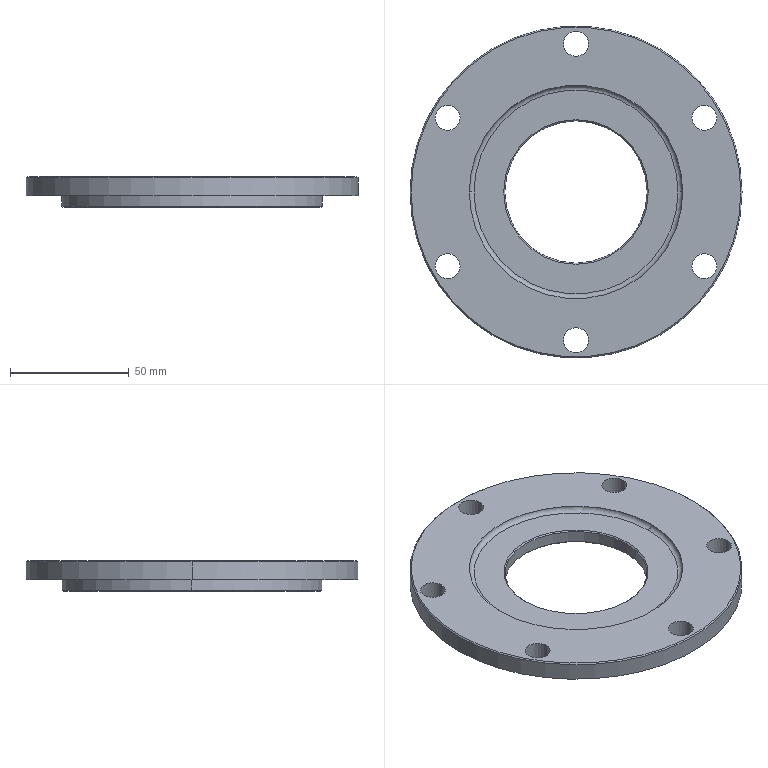Part | SolidWorks | features ICE 3, Chamfer 2, Extrusion 1, Fillet 1 | 1 solid | 35 faces | box 140 x 140 x 13 mm | volume 97648 mm3 | cylinder 20 | cone 8 | plane 5 | torus 2 | commonest cylinder face diameters 10.5 x12 60 x2 100 x2 110 x2 140 x2
STEP:
#1=CARTESIAN_POINT('',(-30.,0.,5.5));
#2=VERTEX_POINT('',#1);
#3=CARTESIAN_POINT('',(30.,0.,5.5));
#4=VERTEX_POINT('',#3);
#5=CARTESIAN_POINT('',(0.,0.,5.5));
#6=DIRECTION('',(0.,0.,1.));
#7=DIRECTION('',(1.,0.,0.));
#8=AXIS2_PLACEMENT_3D('',#5,#6,#7);
#9=CIRCLE('',#8,30.);
#10=EDGE_CURVE('',#2,#4,#9,.T.);
#11=ORIENTED_EDGE('',*,*,#10,.F.);
#12=CARTESIAN_POINT('',(-30.5,0.,6.));
#13=VERTEX_POINT('',#12);
#14=CARTESIAN_POINT('',(-30.,0.,5.5));
#15=DIRECTION('',(-0.7071,0.,0.7071));
#16=VECTOR('',#15,1000.);
#17=LINE('',#14,#16);
#18=EDGE_CURVE('',#2,#13,#17,.T.);
#19=ORIENTED_EDGE('',*,*,#18,.T.);
#20=CARTESIAN_POINT('',(30.5,0.,6.));
#21=VERTEX_POINT('',#20);
#22=CARTESIAN_POINT('',(0.,0.,6.));
#23=DIRECTION('',(0.,0.,-1.));
#24=DIRECTION('',(1.,0.,0.));
#25=AXIS2_PLACEMENT_3D('',#22,#23,#24);
#26=CIRCLE('',#25,30.5);
#27=EDGE_CURVE('',#21,#13,#26,.T.);
#28=ORIENTED_EDGE('',*,*,#27,.F.);
#29=CARTESIAN_POINT('',(30.,0.,5.5));
#30=DIRECTION('',(0.7071,0.,0.7071));
#31=VECTOR('',#30,1000.);
#32=LINE('',#29,#31);
#33=EDGE_CURVE('',#4,#21,#32,.T.);
#34=ORIENTED_EDGE('',*,*,#33,.F.);
#35=EDGE_LOOP('',(#11,#19,#28,#34));
#36=FACE_OUTER_BOUND('',#35,.T.);
#37=CARTESIAN_POINT('',(0.,0.,5.5));
#38=DIRECTION('',(0.,0.,1.));
#39=DIRECTION('',(1.,0.,0.));
#40=AXIS2_PLACEMENT_3D('',#37,#38,#39);
#41=CONICAL_SURFACE('',#40,30.,0.7854);
#42=ADVANCED_FACE('',(#36),#41,.F.);
#43=CARTESIAN_POINT('',(30.,0.,0.5));
#44=VERTEX_POINT('',#43);
#45=CARTESIAN_POINT('',(-30.,0.,0.5));
#46=VERTEX_POINT('',#45);
#47=CARTESIAN_POINT('',(0.,0.,0.5));
#48=DIRECTION('',(0.,0.,-1.));
#49=DIRECTION('',(1.,0.,0.));
#50=AXIS2_PLACEMENT_3D('',#47,#48,#49);
#51=CIRCLE('',#50,30.);
#52=EDGE_CURVE('',#44,#46,#51,.T.);
#53=ORIENTED_EDGE('',*,*,#52,.F.);
#54=CARTESIAN_POINT('',(30.5,0.,0.));
#55=VERTEX_POINT('',#54);
#56=CARTESIAN_POINT('',(30.5,0.,0.));
#57=DIRECTION('',(0.7071,0.,-0.7071));
#58=VECTOR('',#57,1000.);
#59=LINE('',#56,#58);
#60=EDGE_CURVE('',#44,#55,#59,.T.);
#61=ORIENTED_EDGE('',*,*,#60,.T.);
#62=CARTESIAN_POINT('',(-30.5,0.,0.));
#63=VERTEX_POINT('',#62);
#64=CARTESIAN_POINT('',(0.,0.,0.));
#65=DIRECTION('',(0.,0.,1.));
#66=DIRECTION('',(1.,0.,0.));
#67=AXIS2_PLACEMENT_3D('',#64,#65,#66);
#68=CIRCLE('',#67,30.5);
#69=EDGE_CURVE('',#63,#55,#68,.T.);
#70=ORIENTED_EDGE('',*,*,#69,.F.);
#71=CARTESIAN_POINT('',(-30.5,0.,0.));
#72=DIRECTION('',(-0.7071,0.,-0.7071));
#73=VECTOR('',#72,1000.);
#74=LINE('',#71,#73);
#75=EDGE_CURVE('',#46,#63,#74,.T.);
#76=ORIENTED_EDGE('',*,*,#75,.F.);
#77=EDGE_LOOP('',(#53,#61,#70,#76));
#78=FACE_OUTER_BOUND('',#77,.T.);
#79=CARTESIAN_POINT('',(0.,0.,0.));
#80=DIRECTION('',(0.,0.,-1.));
#81=DIRECTION('',(-1.,0.,0.));
#82=AXIS2_PLACEMENT_3D('',#79,#80,#81);
#83=CONICAL_SURFACE('',#82,30.5,0.7854);
#84=ADVANCED_FACE('',(#78),#83,.F.);
#85=ORIENTED_EDGE('',*,*,#52,.T.);
#86=CARTESIAN_POINT('',(-30.,0.,-4.));
#87=DIRECTION('',(0.,0.,1.));
#88=VECTOR('',#87,1000.);
#89=LINE('',#86,#88);
#90=EDGE_CURVE('',#46,#2,#89,.T.);
#91=ORIENTED_EDGE('',*,*,#90,.T.);
#92=ORIENTED_EDGE('',*,*,#10,.T.);
#93=CARTESIAN_POINT('',(30.,0.,-4.));
#94=DIRECTION('',(0.,0.,1.));
#95=VECTOR('',#94,1000.);
#96=LINE('',#93,#95);
#97=EDGE_CURVE('',#44,#4,#96,.T.);
#98=ORIENTED_EDGE('',*,*,#97,.F.);
#99=EDGE_LOOP('',(#85,#91,#92,#98));
#100=FACE_OUTER_BOUND('',#99,.T.);
#101=CARTESIAN_POINT('',(0.,0.,-4.));
#102=DIRECTION('',(0.,0.,1.));
#103=DIRECTION('',(1.,0.,0.));
#104=AXIS2_PLACEMENT_3D('',#101,#102,#103);
#105=CYLINDRICAL_SURFACE('',#104,30.);
#106=ADVANCED_FACE('',(#100),#105,.F.);
#107=CARTESIAN_POINT('',(-43.,0.,6.));
#108=VERTEX_POINT('',#107);
#109=CARTESIAN_POINT('',(43.,0.,6.));
#110=VERTEX_POINT('',#109);
#111=CARTESIAN_POINT('',(0.,0.,6.));
#112=DIRECTION('',(0.,0.,1.));
#113=DIRECTION('',(1.,0.,0.));
#114=AXIS2_PLACEMENT_3D('',#111,#112,#113);
#115=CIRCLE('',#114,43.);
#116=EDGE_CURVE('',#108,#110,#115,.T.);
#117=ORIENTED_EDGE('',*,*,#116,.F.);
#118=CARTESIAN_POINT('',(-45.,0.,8.));
#119=VERTEX_POINT('',#118);
#120=CARTESIAN_POINT('',(-43.,0.,8.));
#121=DIRECTION('',(0.,1.,0.));
#122=DIRECTION('',(-1.,0.,0.));
#123=AXIS2_PLACEMENT_3D('',#120,#121,#122);
#124=CIRCLE('',#123,2.);
#125=EDGE_CURVE('',#108,#119,#124,.T.);
#126=ORIENTED_EDGE('',*,*,#125,.T.);
#127=CARTESIAN_POINT('',(45.,0.,8.));
#128=VERTEX_POINT('',#127);
#129=CARTESIAN_POINT('',(0.,0.,8.));
#130=DIRECTION('',(0.,0.,1.));
#131=DIRECTION('',(1.,0.,0.));
#132=AXIS2_PLACEMENT_3D('',#129,#130,#131);
#133=CIRCLE('',#132,45.);
#134=EDGE_CURVE('',#119,#128,#133,.T.);
#135=ORIENTED_EDGE('',*,*,#134,.T.);
#136=CARTESIAN_POINT('',(43.,0.,8.));
#137=DIRECTION('',(0.,-1.,0.));
#138=DIRECTION('',(0.,0.,-1.));
#139=AXIS2_PLACEMENT_3D('',#136,#137,#138);
#140=CIRCLE('',#139,2.);
#141=EDGE_CURVE('',#110,#128,#140,.T.);
#142=ORIENTED_EDGE('',*,*,#141,.F.);
#143=EDGE_LOOP('',(#117,#126,#135,#142));
#144=FACE_OUTER_BOUND('',#143,.T.);
#145=CARTESIAN_POINT('',(0.,0.,8.));
#146=DIRECTION('',(0.,0.,1.));
#147=DIRECTION('',(1.,0.,0.));
#148=AXIS2_PLACEMENT_3D('',#145,#146,#147);
#149=TOROIDAL_SURFACE('',#148,43.,2.);
#150=ADVANCED_FACE('',(#144),#149,.F.);
#151=CARTESIAN_POINT('',(69.5,0.,8.));
#152=VERTEX_POINT('',#151);
#153=CARTESIAN_POINT('',(-69.5,0.,8.));
#154=VERTEX_POINT('',#153);
#155=CARTESIAN_POINT('',(0.,0.,8.));
#156=DIRECTION('',(0.,0.,1.));
#157=DIRECTION('',(1.,0.,0.));
#158=AXIS2_PLACEMENT_3D('',#155,#156,#157);
#159=CIRCLE('',#158,69.5);
#160=EDGE_CURVE('',#152,#154,#159,.T.);
#161=ORIENTED_EDGE('',*,*,#160,.F.);
#162=CARTESIAN_POINT('',(70.,0.,7.5));
#163=VERTEX_POINT('',#162);
#164=CARTESIAN_POINT('',(69.5,0.,8.));
#165=DIRECTION('',(0.7071,0.,-0.7071));
#166=VECTOR('',#165,1000.);
#167=LINE('',#164,#166);
#168=EDGE_CURVE('',#152,#163,#167,.T.);
#169=ORIENTED_EDGE('',*,*,#168,.T.);
#170=CARTESIAN_POINT('',(-70.,0.,7.5));
#171=VERTEX_POINT('',#170);
#172=CARTESIAN_POINT('',(0.,0.,7.5));
#173=DIRECTION('',(0.,0.,-1.));
#174=DIRECTION('',(1.,0.,0.));
#175=AXIS2_PLACEMENT_3D('',#172,#173,#174);
#176=CIRCLE('',#175,70.);
#177=EDGE_CURVE('',#171,#163,#176,.T.);
#178=ORIENTED_EDGE('',*,*,#177,.F.);
#179=CARTESIAN_POINT('',(-69.5,0.,8.));
#180=DIRECTION('',(-0.7071,0.,-0.7071));
#181=VECTOR('',#180,1000.);
#182=LINE('',#179,#181);
#183=EDGE_CURVE('',#154,#171,#182,.T.);
#184=ORIENTED_EDGE('',*,*,#183,.F.);
#185=EDGE_LOOP('',(#161,#169,#178,#184));
#186=FACE_OUTER_BOUND('',#185,.T.);
#187=CARTESIAN_POINT('',(0.,0.,8.));
#188=DIRECTION('',(0.,0.,-1.));
#189=DIRECTION('',(-1.,0.,0.));
#190=AXIS2_PLACEMENT_3D('',#187,#188,#189);
#191=CONICAL_SURFACE('',#190,69.5,0.7854);
#192=ADVANCED_FACE('',(#186),#191,.T.);
#193=CARTESIAN_POINT('',(-54.5,0.,-5.));
#194=VERTEX_POINT('',#193);
#195=CARTESIAN_POINT('',(54.5,0.,-5.));
#196=VERTEX_POINT('',#195);
#197=CARTESIAN_POINT('',(0.,0.,-5.));
#198=DIRECTION('',(0.,0.,-1.));
#199=DIRECTION('',(-1.,0.,0.));
#200=AXIS2_PLACEMENT_3D('',#197,#198,#199);
#201=CIRCLE('',#200,54.5);
#202=EDGE_CURVE('',#194,#196,#201,.T.);
#203=ORIENTED_EDGE('',*,*,#202,.F.);
#204=CARTESIAN_POINT('',(-55.,0.,-4.5));
#205=VERTEX_POINT('',#204);
#206=CARTESIAN_POINT('',(-54.5,0.,-5.));
#207=DIRECTION('',(-0.7071,0.,0.7071));
#208=VECTOR('',#207,1000.);
#209=LINE('',#206,#208);
#210=EDGE_CURVE('',#194,#205,#209,.T.);
#211=ORIENTED_EDGE('',*,*,#210,.T.);
#212=CARTESIAN_POINT('',(55.,0.,-4.5));
#213=VERTEX_POINT('',#212);
#214=CARTESIAN_POINT('',(0.,0.,-4.5));
#215=DIRECTION('',(0.,0.,1.));
#216=DIRECTION('',(-1.,0.,0.));
#217=AXIS2_PLACEMENT_3D('',#214,#215,#216);
#218=CIRCLE('',#217,55.);
#219=EDGE_CURVE('',#213,#205,#218,.T.);
#220=ORIENTED_EDGE('',*,*,#219,.F.);
#221=CARTESIAN_POINT('',(54.5,0.,-5.));
#222=DIRECTION('',(0.7071,0.,0.7071));
#223=VECTOR('',#222,1000.);
#224=LINE('',#221,#223);
#225=EDGE_CURVE('',#196,#213,#224,.T.);
#226=ORIENTED_EDGE('',*,*,#225,.F.);
#227=EDGE_LOOP('',(#203,#211,#220,#226));
#228=FACE_OUTER_BOUND('',#227,.T.);
#229=CARTESIAN_POINT('',(0.,0.,-5.));
#230=DIRECTION('',(0.,0.,1.));
#231=DIRECTION('',(1.,0.,0.));
#232=AXIS2_PLACEMENT_3D('',#229,#230,#231);
#233=CONICAL_SURFACE('',#232,54.5,0.7854);
#234=ADVANCED_FACE('',(#228),#233,.T.);
#235=CARTESIAN_POINT('',(50.,0.,-5.));
#236=VERTEX_POINT('',#235);
#237=CARTESIAN_POINT('',(-50.,0.,-5.));
#238=VERTEX_POINT('',#237);
#239=CARTESIAN_POINT('',(0.,0.,-5.));
#240=DIRECTION('',(0.,0.,-1.));
#241=DIRECTION('',(-1.,0.,0.));
#242=AXIS2_PLACEMENT_3D('',#239,#240,#241);
#243=CIRCLE('',#242,50.);
#244=EDGE_CURVE('',#236,#238,#243,.T.);
#245=ORIENTED_EDGE('',*,*,#244,.T.);
#246=CARTESIAN_POINT('',(-50.,0.,0.));
#247=VERTEX_POINT('',#246);
#248=CARTESIAN_POINT('',(-50.,0.,-5.));
#249=DIRECTION('',(0.,0.,1.));
#250=VECTOR('',#249,1000.);
#251=LINE('',#248,#250);
#252=EDGE_CURVE('',#238,#247,#251,.T.);
#253=ORIENTED_EDGE('',*,*,#252,.T.);
#254=CARTESIAN_POINT('',(50.,0.,0.));
#255=VERTEX_POINT('',#254);
#256=CARTESIAN_POINT('',(0.,0.,0.));
#257=DIRECTION('',(0.,0.,-1.));
#258=DIRECTION('',(-1.,0.,0.));
#259=AXIS2_PLACEMENT_3D('',#256,#257,#258);
#260=CIRCLE('',#259,50.);
#261=EDGE_CURVE('',#255,#247,#260,.T.);
#262=ORIENTED_EDGE('',*,*,#261,.F.);
#263=CARTESIAN_POINT('',(50.,0.,-5.));
#264=DIRECTION('',(0.,0.,1.));
#265=VECTOR('',#264,1000.);
#266=LINE('',#263,#265);
#267=EDGE_CURVE('',#236,#255,#266,.T.);
#268=ORIENTED_EDGE('',*,*,#267,.F.);
#269=EDGE_LOOP('',(#245,#253,#262,#268));
#270=FACE_OUTER_BOUND('',#269,.T.);
#271=CARTESIAN_POINT('',(0.,0.,-5.));
#272=DIRECTION('',(0.,0.,1.));
#273=DIRECTION('',(1.,0.,0.));
#274=AXIS2_PLACEMENT_3D('',#271,#272,#273);
#275=CYLINDRICAL_SURFACE('',#274,50.);
#276=ADVANCED_FACE('',(#270),#275,.F.);
#277=ORIENTED_EDGE('',*,*,#219,.T.);
#278=CARTESIAN_POINT('',(-55.,0.,0.));
#279=VERTEX_POINT('',#278);
#280=CARTESIAN_POINT('',(-55.,0.,-5.));
#281=DIRECTION('',(0.,0.,1.));
#282=VECTOR('',#281,1000.);
#283=LINE('',#280,#282);
#284=EDGE_CURVE('',#205,#279,#283,.T.);
#285=ORIENTED_EDGE('',*,*,#284,.T.);
#286=CARTESIAN_POINT('',(55.,0.,0.));
#287=VERTEX_POINT('',#286);
#288=CARTESIAN_POINT('',(0.,0.,0.));
#289=DIRECTION('',(0.,0.,-1.));
#290=DIRECTION('',(1.,0.,0.));
#291=AXIS2_PLACEMENT_3D('',#288,#289,#290);
#292=CIRCLE('',#291,55.);
#293=EDGE_CURVE('',#279,#287,#292,.T.);
#294=ORIENTED_EDGE('',*,*,#293,.T.);
#295=CARTESIAN_POINT('',(55.,0.,-5.));
#296=DIRECTION('',(0.,0.,1.));
#297=VECTOR('',#296,1000.);
#298=LINE('',#295,#297);
#299=EDGE_CURVE('',#213,#287,#298,.T.);
#300=ORIENTED_EDGE('',*,*,#299,.F.);
#301=EDGE_LOOP('',(#277,#285,#294,#300));
#302=FACE_OUTER_BOUND('',#301,.T.);
#303=CARTESIAN_POINT('',(0.,0.,-5.));
#304=DIRECTION('',(0.,0.,1.));
#305=DIRECTION('',(1.,0.,0.));
#306=AXIS2_PLACEMENT_3D('',#303,#304,#305);
#307=CYLINDRICAL_SURFACE('',#306,55.);
#308=ADVANCED_FACE('',(#302),#307,.T.);
#309=CARTESIAN_POINT('',(-59.377,31.25,8.));
#310=VERTEX_POINT('',#309);
#311=CARTESIAN_POINT('',(-48.877,31.25,8.));
#312=VERTEX_POINT('',#311);
#313=CARTESIAN_POINT('',(-54.127,31.25,8.));
#314=DIRECTION('',(0.,0.,1.));
#315=DIRECTION('',(1.,0.,0.));
#316=AXIS2_PLACEMENT_3D('',#313,#314,#315);
#317=CIRCLE('',#316,5.25);
#318=EDGE_CURVE('',#310,#312,#317,.T.);
#319=ORIENTED_EDGE('',*,*,#318,.T.);
#320=CARTESIAN_POINT('',(-48.877,31.25,0.));
#321=VERTEX_POINT('',#320);
#322=CARTESIAN_POINT('',(-48.877,31.25,8.));
#323=DIRECTION('',(0.,0.,-1.));
#324=VECTOR('',#323,1000.);
#325=LINE('',#322,#324);
#326=EDGE_CURVE('',#312,#321,#325,.T.);
#327=ORIENTED_EDGE('',*,*,#326,.T.);
#328=CARTESIAN_POINT('',(-59.377,31.25,0.));
#329=VERTEX_POINT('',#328);
#330=CARTESIAN_POINT('',(-54.127,31.25,0.));
#331=DIRECTION('',(0.,0.,1.));
#332=DIRECTION('',(1.,0.,0.));
#333=AXIS2_PLACEMENT_3D('',#330,#331,#332);
#334=CIRCLE('',#333,5.25);
#335=EDGE_CURVE('',#329,#321,#334,.T.);
#336=ORIENTED_EDGE('',*,*,#335,.F.);
#337=CARTESIAN_POINT('',(-59.377,31.25,8.));
#338=DIRECTION('',(0.,0.,-1.));
#339=VECTOR('',#338,1000.);
#340=LINE('',#337,#339);
#341=EDGE_CURVE('',#310,#329,#340,.T.);
#342=ORIENTED_EDGE('',*,*,#341,.F.);
#343=EDGE_LOOP('',(#319,#327,#336,#342));
#344=FACE_OUTER_BOUND('',#343,.T.);
#345=CARTESIAN_POINT('',(-54.127,31.25,8.));
#346=DIRECTION('',(0.,0.,-1.));
#347=DIRECTION('',(-1.,0.,0.));
#348=AXIS2_PLACEMENT_3D('',#345,#346,#347);
#349=CYLINDRICAL_SURFACE('',#348,5.25);
#350=ADVANCED_FACE('',(#344),#349,.F.);
#351=CARTESIAN_POINT('',(-59.377,-31.25,8.));
#352=VERTEX_POINT('',#351);
#353=CARTESIAN_POINT('',(-48.877,-31.25,8.));
#354=VERTEX_POINT('',#353);
#355=CARTESIAN_POINT('',(-54.127,-31.25,8.));
#356=DIRECTION('',(0.,0.,1.));
#357=DIRECTION('',(1.,0.,0.));
#358=AXIS2_PLACEMENT_3D('',#355,#356,#357);
#359=CIRCLE('',#358,5.25);
#360=EDGE_CURVE('',#352,#354,#359,.T.);
#361=ORIENTED_EDGE('',*,*,#360,.T.);
#362=CARTESIAN_POINT('',(-48.877,-31.25,0.));
#363=VERTEX_POINT('',#362);
#364=CARTESIAN_POINT('',(-48.877,-31.25,8.));
#365=DIRECTION('',(0.,0.,-1.));
#366=VECTOR('',#365,1000.);
#367=LINE('',#364,#366);
#368=EDGE_CURVE('',#354,#363,#367,.T.);
#369=ORIENTED_EDGE('',*,*,#368,.T.);
#370=CARTESIAN_POINT('',(-59.377,-31.25,0.));
#371=VERTEX_POINT('',#370);
#372=CARTESIAN_POINT('',(-54.127,-31.25,0.));
#373=DIRECTION('',(0.,0.,1.));
#374=DIRECTION('',(1.,0.,0.));
#375=AXIS2_PLACEMENT_3D('',#372,#373,#374);
#376=CIRCLE('',#375,5.25);
#377=EDGE_CURVE('',#371,#363,#376,.T.);
#378=ORIENTED_EDGE('',*,*,#377,.F.);
#379=CARTESIAN_POINT('',(-59.377,-31.25,8.));
#380=DIRECTION('',(0.,0.,-1.));
#381=VECTOR('',#380,1000.);
#382=LINE('',#379,#381);
#383=EDGE_CURVE('',#352,#371,#382,.T.);
#384=ORIENTED_EDGE('',*,*,#383,.F.);
#385=EDGE_LOOP('',(#361,#369,#378,#384));
#386=FACE_OUTER_BOUND('',#385,.T.);
#387=CARTESIAN_POINT('',(-54.127,-31.25,8.));
#388=DIRECTION('',(0.,0.,-1.));
#389=DIRECTION('',(-1.,0.,0.));
#390=AXIS2_PLACEMENT_3D('',#387,#388,#389);
#391=CYLINDRICAL_SURFACE('',#390,5.25);
#392=ADVANCED_FACE('',(#386),#391,.F.);
#393=CARTESIAN_POINT('',(-5.25,-62.5,8.));
#394=VERTEX_POINT('',#393);
#395=CARTESIAN_POINT('',(5.25,-62.5,8.));
#396=VERTEX_POINT('',#395);
#397=CARTESIAN_POINT('',(0.,-62.5,8.));
#398=DIRECTION('',(0.,0.,1.));
#399=DIRECTION('',(1.,0.,0.));
#400=AXIS2_PLACEMENT_3D('',#397,#398,#399);
#401=CIRCLE('',#400,5.25);
#402=EDGE_CURVE('',#394,#396,#401,.T.);
#403=ORIENTED_EDGE('',*,*,#402,.T.);
#404=CARTESIAN_POINT('',(5.25,-62.5,0.));
#405=VERTEX_POINT('',#404);
#406=CARTESIAN_POINT('',(5.25,-62.5,8.));
#407=DIRECTION('',(0.,0.,-1.));
#408=VECTOR('',#407,1000.);
#409=LINE('',#406,#408);
#410=EDGE_CURVE('',#396,#405,#409,.T.);
#411=ORIENTED_EDGE('',*,*,#410,.T.);
#412=CARTESIAN_POINT('',(-5.25,-62.5,0.));
#413=VERTEX_POINT('',#412);
#414=CARTESIAN_POINT('',(0.,-62.5,0.));
#415=DIRECTION('',(0.,0.,1.));
#416=DIRECTION('',(1.,0.,0.));
#417=AXIS2_PLACEMENT_3D('',#414,#415,#416);
#418=CIRCLE('',#417,5.25);
#419=EDGE_CURVE('',#413,#405,#418,.T.);
#420=ORIENTED_EDGE('',*,*,#419,.F.);
#421=CARTESIAN_POINT('',(-5.25,-62.5,8.));
#422=DIRECTION('',(0.,0.,-1.));
#423=VECTOR('',#422,1000.);
#424=LINE('',#421,#423);
#425=EDGE_CURVE('',#394,#413,#424,.T.);
#426=ORIENTED_EDGE('',*,*,#425,.F.);
#427=EDGE_LOOP('',(#403,#411,#420,#426));
#428=FACE_OUTER_BOUND('',#427,.T.);
#429=CARTESIAN_POINT('',(0.,-62.5,8.));
#430=DIRECTION('',(0.,0.,-1.));
#431=DIRECTION('',(-1.,0.,0.));
#432=AXIS2_PLACEMENT_3D('',#429,#430,#431);
#433=CYLINDRICAL_SURFACE('',#432,5.25);
#434=ADVANCED_FACE('',(#428),#433,.F.);
#435=CARTESIAN_POINT('',(48.877,-31.25,8.));
#436=VERTEX_POINT('',#435);
#437=CARTESIAN_POINT('',(59.377,-31.25,8.));
#438=VERTEX_POINT('',#437);
#439=CARTESIAN_POINT('',(54.127,-31.25,8.));
#440=DIRECTION('',(0.,0.,1.));
#441=DIRECTION('',(1.,0.,0.));
#442=AXIS2_PLACEMENT_3D('',#439,#440,#441);
#443=CIRCLE('',#442,5.25);
#444=EDGE_CURVE('',#436,#438,#443,.T.);
#445=ORIENTED_EDGE('',*,*,#444,.T.);
#446=CARTESIAN_POINT('',(59.377,-31.25,0.));
#447=VERTEX_POINT('',#446);
#448=CARTESIAN_POINT('',(59.377,-31.25,8.));
#449=DIRECTION('',(0.,0.,-1.));
#450=VECTOR('',#449,1000.);
#451=LINE('',#448,#450);
#452=EDGE_CURVE('',#438,#447,#451,.T.);
#453=ORIENTED_EDGE('',*,*,#452,.T.);
#454=CARTESIAN_POINT('',(48.877,-31.25,0.));
#455=VERTEX_POINT('',#454);
#456=CARTESIAN_POINT('',(54.127,-31.25,0.));
#457=DIRECTION('',(0.,0.,1.));
#458=DIRECTION('',(1.,0.,0.));
#459=AXIS2_PLACEMENT_3D('',#456,#457,#458);
#460=CIRCLE('',#459,5.25);
#461=EDGE_CURVE('',#455,#447,#460,.T.);
#462=ORIENTED_EDGE('',*,*,#461,.F.);
#463=CARTESIAN_POINT('',(48.877,-31.25,8.));
#464=DIRECTION('',(0.,0.,-1.));
#465=VECTOR('',#464,1000.);
#466=LINE('',#463,#465);
#467=EDGE_CURVE('',#436,#455,#466,.T.);
#468=ORIENTED_EDGE('',*,*,#467,.F.);
#469=EDGE_LOOP('',(#445,#453,#462,#468));
#470=FACE_OUTER_BOUND('',#469,.T.);
#471=CARTESIAN_POINT('',(54.127,-31.25,8.));
#472=DIRECTION('',(0.,0.,-1.));
#473=DIRECTION('',(-1.,0.,0.));
#474=AXIS2_PLACEMENT_3D('',#471,#472,#473);
#475=CYLINDRICAL_SURFACE('',#474,5.25);
#476=ADVANCED_FACE('',(#470),#475,.F.);
#477=CARTESIAN_POINT('',(48.877,31.25,8.));
#478=VERTEX_POINT('',#477);
#479=CARTESIAN_POINT('',(59.377,31.25,8.));
#480=VERTEX_POINT('',#479);
#481=CARTESIAN_POINT('',(54.127,31.25,8.));
#482=DIRECTION('',(0.,0.,1.));
#483=DIRECTION('',(1.,0.,0.));
#484=AXIS2_PLACEMENT_3D('',#481,#482,#483);
#485=CIRCLE('',#484,5.25);
#486=EDGE_CURVE('',#478,#480,#485,.T.);
#487=ORIENTED_EDGE('',*,*,#486,.T.);
#488=CARTESIAN_POINT('',(59.377,31.25,0.));
#489=VERTEX_POINT('',#488);
#490=CARTESIAN_POINT('',(59.377,31.25,8.));
#491=DIRECTION('',(0.,0.,-1.));
#492=VECTOR('',#491,1000.);
#493=LINE('',#490,#492);
#494=EDGE_CURVE('',#480,#489,#493,.T.);
#495=ORIENTED_EDGE('',*,*,#494,.T.);
#496=CARTESIAN_POINT('',(48.877,31.25,0.));
#497=VERTEX_POINT('',#496);
#498=CARTESIAN_POINT('',(54.127,31.25,0.));
#499=DIRECTION('',(0.,0.,1.));
#500=DIRECTION('',(1.,0.,0.));
#501=AXIS2_PLACEMENT_3D('',#498,#499,#500);
#502=CIRCLE('',#501,5.25);
#503=EDGE_CURVE('',#497,#489,#502,.T.);
#504=ORIENTED_EDGE('',*,*,#503,.F.);
#505=CARTESIAN_POINT('',(48.877,31.25,8.));
#506=DIRECTION('',(0.,0.,-1.));
#507=VECTOR('',#506,1000.);
#508=LINE('',#505,#507);
#509=EDGE_CURVE('',#478,#497,#508,.T.);
#510=ORIENTED_EDGE('',*,*,#509,.F.);
#511=EDGE_LOOP('',(#487,#495,#504,#510));
#512=FACE_OUTER_BOUND('',#511,.T.);
#513=CARTESIAN_POINT('',(54.127,31.25,8.));
#514=DIRECTION('',(0.,0.,-1.));
#515=DIRECTION('',(-1.,0.,0.));
#516=AXIS2_PLACEMENT_3D('',#513,#514,#515);
#517=CYLINDRICAL_SURFACE('',#516,5.25);
#518=ADVANCED_FACE('',(#512),#517,.F.);
#519=CARTESIAN_POINT('',(-5.25,62.5,8.));
#520=VERTEX_POINT('',#519);
#521=CARTESIAN_POINT('',(5.25,62.5,8.));
#522=VERTEX_POINT('',#521);
#523=CARTESIAN_POINT('',(0.,62.5,8.));
#524=DIRECTION('',(0.,0.,1.));
#525=DIRECTION('',(1.,0.,0.));
#526=AXIS2_PLACEMENT_3D('',#523,#524,#525);
#527=CIRCLE('',#526,5.25);
#528=EDGE_CURVE('',#520,#522,#527,.T.);
#529=ORIENTED_EDGE('',*,*,#528,.T.);
#530=CARTESIAN_POINT('',(5.25,62.5,0.));
#531=VERTEX_POINT('',#530);
#532=CARTESIAN_POINT('',(5.25,62.5,8.));
#533=DIRECTION('',(0.,0.,-1.));
#534=VECTOR('',#533,1000.);
#535=LINE('',#532,#534);
#536=EDGE_CURVE('',#522,#531,#535,.T.);
#537=ORIENTED_EDGE('',*,*,#536,.T.);
#538=CARTESIAN_POINT('',(-5.25,62.5,0.));
#539=VERTEX_POINT('',#538);
#540=CARTESIAN_POINT('',(0.,62.5,0.));
#541=DIRECTION('',(0.,0.,1.));
#542=DIRECTION('',(1.,0.,0.));
#543=AXIS2_PLACEMENT_3D('',#540,#541,#542);
#544=CIRCLE('',#543,5.25);
#545=EDGE_CURVE('',#539,#531,#544,.T.);
#546=ORIENTED_EDGE('',*,*,#545,.F.);
#547=CARTESIAN_POINT('',(-5.25,62.5,8.));
#548=DIRECTION('',(0.,0.,-1.));
#549=VECTOR('',#548,1000.);
#550=LINE('',#547,#549);
#551=EDGE_CURVE('',#520,#539,#550,.T.);
#552=ORIENTED_EDGE('',*,*,#551,.F.);
#553=EDGE_LOOP('',(#529,#537,#546,#552));
#554=FACE_OUTER_BOUND('',#553,.T.);
#555=CARTESIAN_POINT('',(0.,62.5,8.));
#556=DIRECTION('',(0.,0.,-1.));
#557=DIRECTION('',(-1.,0.,0.));
#558=AXIS2_PLACEMENT_3D('',#555,#556,#557);
#559=CYLINDRICAL_SURFACE('',#558,5.25);
#560=ADVANCED_FACE('',(#554),#559,.F.);
#561=ORIENTED_EDGE('',*,*,#177,.T.);
#562=CARTESIAN_POINT('',(70.,0.,0.));
#563=VERTEX_POINT('',#562);
#564=CARTESIAN_POINT('',(70.,0.,8.));
#565=DIRECTION('',(0.,0.,-1.));
#566=VECTOR('',#565,1000.);
#567=LINE('',#564,#566);
#568=EDGE_CURVE('',#163,#563,#567,.T.);
#569=ORIENTED_EDGE('',*,*,#568,.T.);
#570=CARTESIAN_POINT('',(-70.,0.,0.));
#571=VERTEX_POINT('',#570);
#572=CARTESIAN_POINT('',(0.,0.,0.));
#573=DIRECTION('',(0.,0.,1.));
#574=DIRECTION('',(1.,0.,0.));
#575=AXIS2_PLACEMENT_3D('',#572,#573,#574);
#576=CIRCLE('',#575,70.);
#577=EDGE_CURVE('',#563,#571,#576,.T.);
#578=ORIENTED_EDGE('',*,*,#577,.T.);
#579=CARTESIAN_POINT('',(-70.,0.,8.));
#580=DIRECTION('',(0.,0.,-1.));
#581=VECTOR('',#580,1000.);
#582=LINE('',#579,#581);
#583=EDGE_CURVE('',#171,#571,#582,.T.);
#584=ORIENTED_EDGE('',*,*,#583,.F.);
#585=EDGE_LOOP('',(#561,#569,#578,#584));
#586=FACE_OUTER_BOUND('',#585,.T.);
#587=CARTESIAN_POINT('',(0.,0.,8.));
#588=DIRECTION('',(0.,0.,-1.));
#589=DIRECTION('',(-1.,0.,0.));
#590=AXIS2_PLACEMENT_3D('',#587,#588,#589);
#591=CYLINDRICAL_SURFACE('',#590,70.);
#592=ADVANCED_FACE('',(#586),#591,.T.);
#593=CARTESIAN_POINT('',(0.,0.,8.));
#594=DIRECTION('',(0.,0.,1.));
#595=DIRECTION('',(1.,0.,0.));
#596=AXIS2_PLACEMENT_3D('',#593,#594,#595);
#597=CIRCLE('',#596,45.);
#598=EDGE_CURVE('',#128,#119,#597,.T.);
#599=ORIENTED_EDGE('',*,*,#598,.F.);
#600=ORIENTED_EDGE('',*,*,#134,.F.);
#601=EDGE_LOOP('',(#599,#600));
#602=FACE_BOUND('',#601,.T.);
#603=CARTESIAN_POINT('',(0.,0.,8.));
#604=DIRECTION('',(0.,0.,1.));
#605=DIRECTION('',(1.,0.,0.));
#606=AXIS2_PLACEMENT_3D('',#603,#604,#605);
#607=CIRCLE('',#606,69.5);
#608=EDGE_CURVE('',#154,#152,#607,.T.);
#609=ORIENTED_EDGE('',*,*,#608,.T.);
#610=ORIENTED_EDGE('',*,*,#160,.T.);
#611=EDGE_LOOP('',(#609,#610));
#612=FACE_OUTER_BOUND('',#611,.T.);
#613=ORIENTED_EDGE('',*,*,#360,.F.);
#614=CARTESIAN_POINT('',(-54.127,-31.25,8.));
#615=DIRECTION('',(0.,0.,1.));
#616=DIRECTION('',(1.,0.,0.));
#617=AXIS2_PLACEMENT_3D('',#614,#615,#616);
#618=CIRCLE('',#617,5.25);
#619=EDGE_CURVE('',#354,#352,#618,.T.);
#620=ORIENTED_EDGE('',*,*,#619,.F.);
#621=EDGE_LOOP('',(#613,#620));
#622=FACE_BOUND('',#621,.T.);
#623=ORIENTED_EDGE('',*,*,#444,.F.);
#624=CARTESIAN_POINT('',(54.127,-31.25,8.));
#625=DIRECTION('',(0.,0.,1.));
#626=DIRECTION('',(1.,0.,0.));
#627=AXIS2_PLACEMENT_3D('',#624,#625,#626);
#628=CIRCLE('',#627,5.25);
#629=EDGE_CURVE('',#438,#436,#628,.T.);
#630=ORIENTED_EDGE('',*,*,#629,.F.);
#631=EDGE_LOOP('',(#623,#630));
#632=FACE_BOUND('',#631,.T.);
#633=ORIENTED_EDGE('',*,*,#528,.F.);
#634=CARTESIAN_POINT('',(0.,62.5,8.));
#635=DIRECTION('',(0.,0.,1.));
#636=DIRECTION('',(1.,0.,0.));
#637=AXIS2_PLACEMENT_3D('',#634,#635,#636);
#638=CIRCLE('',#637,5.25);
#639=EDGE_CURVE('',#522,#520,#638,.T.);
#640=ORIENTED_EDGE('',*,*,#639,.F.);
#641=EDGE_LOOP('',(#633,#640));
#642=FACE_BOUND('',#641,.T.);
#643=ORIENTED_EDGE('',*,*,#486,.F.);
#644=CARTESIAN_POINT('',(54.127,31.25,8.));
#645=DIRECTION('',(0.,0.,1.));
#646=DIRECTION('',(1.,0.,0.));
#647=AXIS2_PLACEMENT_3D('',#644,#645,#646);
#648=CIRCLE('',#647,5.25);
#649=EDGE_CURVE('',#480,#478,#648,.T.);
#650=ORIENTED_EDGE('',*,*,#649,.F.);
#651=EDGE_LOOP('',(#643,#650));
#652=FACE_BOUND('',#651,.T.);
#653=ORIENTED_EDGE('',*,*,#402,.F.);
#654=CARTESIAN_POINT('',(0.,-62.5,8.));
#655=DIRECTION('',(0.,0.,1.));
#656=DIRECTION('',(1.,0.,0.));
#657=AXIS2_PLACEMENT_3D('',#654,#655,#656);
#658=CIRCLE('',#657,5.25);
#659=EDGE_CURVE('',#396,#394,#658,.T.);
#660=ORIENTED_EDGE('',*,*,#659,.F.);
#661=EDGE_LOOP('',(#653,#660));
#662=FACE_BOUND('',#661,.T.);
#663=ORIENTED_EDGE('',*,*,#318,.F.);
#664=CARTESIAN_POINT('',(-54.127,31.25,8.));
#665=DIRECTION('',(0.,0.,1.));
#666=DIRECTION('',(1.,0.,0.));
#667=AXIS2_PLACEMENT_3D('',#664,#665,#666);
#668=CIRCLE('',#667,5.25);
#669=EDGE_CURVE('',#312,#310,#668,.T.);
#670=ORIENTED_EDGE('',*,*,#669,.F.);
#671=EDGE_LOOP('',(#663,#670));
#672=FACE_BOUND('',#671,.T.);
#673=CARTESIAN_POINT('',(0.,0.,8.));
#674=DIRECTION('',(0.,0.,1.));
#675=DIRECTION('',(1.,0.,0.));
#676=AXIS2_PLACEMENT_3D('',#673,#674,#675);
#677=PLANE('',#676);
#678=ADVANCED_FACE('',(#602,#612,#622,#632,#642,#652,#662,#672),#677,.T.);
#679=CARTESIAN_POINT('',(0.,0.,0.));
#680=DIRECTION('',(0.,0.,-1.));
#681=DIRECTION('',(1.,0.,0.));
#682=AXIS2_PLACEMENT_3D('',#679,#680,#681);
#683=CIRCLE('',#682,55.);
#684=EDGE_CURVE('',#287,#279,#683,.T.);
#685=ORIENTED_EDGE('',*,*,#684,.F.);
#686=ORIENTED_EDGE('',*,*,#293,.F.);
#687=EDGE_LOOP('',(#685,#686));
#688=FACE_BOUND('',#687,.T.);
#689=CARTESIAN_POINT('',(0.,0.,0.));
#690=DIRECTION('',(0.,0.,1.));
#691=DIRECTION('',(1.,0.,0.));
#692=AXIS2_PLACEMENT_3D('',#689,#690,#691);
#693=CIRCLE('',#692,70.);
#694=EDGE_CURVE('',#571,#563,#693,.T.);
#695=ORIENTED_EDGE('',*,*,#694,.F.);
#696=ORIENTED_EDGE('',*,*,#577,.F.);
#697=EDGE_LOOP('',(#695,#696));
#698=FACE_OUTER_BOUND('',#697,.T.);
#699=ORIENTED_EDGE('',*,*,#545,.T.);
#700=CARTESIAN_POINT('',(0.,62.5,0.));
#701=DIRECTION('',(0.,0.,1.));
#702=DIRECTION('',(1.,0.,0.));
#703=AXIS2_PLACEMENT_3D('',#700,#701,#702);
#704=CIRCLE('',#703,5.25);
#705=EDGE_CURVE('',#531,#539,#704,.T.);
#706=ORIENTED_EDGE('',*,*,#705,.T.);
#707=EDGE_LOOP('',(#699,#706));
#708=FACE_BOUND('',#707,.T.);
#709=ORIENTED_EDGE('',*,*,#503,.T.);
#710=CARTESIAN_POINT('',(54.127,31.25,0.));
#711=DIRECTION('',(0.,0.,1.));
#712=DIRECTION('',(1.,0.,0.));
#713=AXIS2_PLACEMENT_3D('',#710,#711,#712);
#714=CIRCLE('',#713,5.25);
#715=EDGE_CURVE('',#489,#497,#714,.T.);
#716=ORIENTED_EDGE('',*,*,#715,.T.);
#717=EDGE_LOOP('',(#709,#716));
#718=FACE_BOUND('',#717,.T.);
#719=ORIENTED_EDGE('',*,*,#461,.T.);
#720=CARTESIAN_POINT('',(54.127,-31.25,0.));
#721=DIRECTION('',(0.,0.,1.));
#722=DIRECTION('',(1.,0.,0.));
#723=AXIS2_PLACEMENT_3D('',#720,#721,#722);
#724=CIRCLE('',#723,5.25);
#725=EDGE_CURVE('',#447,#455,#724,.T.);
#726=ORIENTED_EDGE('',*,*,#725,.T.);
#727=EDGE_LOOP('',(#719,#726));
#728=FACE_BOUND('',#727,.T.);
#729=ORIENTED_EDGE('',*,*,#419,.T.);
#730=CARTESIAN_POINT('',(0.,-62.5,0.));
#731=DIRECTION('',(0.,0.,1.));
#732=DIRECTION('',(1.,0.,0.));
#733=AXIS2_PLACEMENT_3D('',#730,#731,#732);
#734=CIRCLE('',#733,5.25);
#735=EDGE_CURVE('',#405,#413,#734,.T.);
#736=ORIENTED_EDGE('',*,*,#735,.T.);
#737=EDGE_LOOP('',(#729,#736));
#738=FACE_BOUND('',#737,.T.);
#739=ORIENTED_EDGE('',*,*,#377,.T.);
#740=CARTESIAN_POINT('',(-54.127,-31.25,0.));
#741=DIRECTION('',(0.,0.,1.));
#742=DIRECTION('',(1.,0.,0.));
#743=AXIS2_PLACEMENT_3D('',#740,#741,#742);
#744=CIRCLE('',#743,5.25);
#745=EDGE_CURVE('',#363,#371,#744,.T.);
#746=ORIENTED_EDGE('',*,*,#745,.T.);
#747=EDGE_LOOP('',(#739,#746));
#748=FACE_BOUND('',#747,.T.);
#749=ORIENTED_EDGE('',*,*,#335,.T.);
#750=CARTESIAN_POINT('',(-54.127,31.25,0.));
#751=DIRECTION('',(0.,0.,1.));
#752=DIRECTION('',(1.,0.,0.));
#753=AXIS2_PLACEMENT_3D('',#750,#751,#752);
#754=CIRCLE('',#753,5.25);
#755=EDGE_CURVE('',#321,#329,#754,.T.);
#756=ORIENTED_EDGE('',*,*,#755,.T.);
#757=EDGE_LOOP('',(#749,#756));
#758=FACE_BOUND('',#757,.T.);
#759=CARTESIAN_POINT('',(0.,0.,0.));
#760=DIRECTION('',(0.,0.,1.));
#761=DIRECTION('',(1.,0.,0.));
#762=AXIS2_PLACEMENT_3D('',#759,#760,#761);
#763=PLANE('',#762);
#764=ADVANCED_FACE('',(#688,#698,#708,#718,#728,#738,#748,#758),#763,.F.);
#765=ORIENTED_EDGE('',*,*,#568,.F.);
#766=CARTESIAN_POINT('',(0.,0.,7.5));
#767=DIRECTION('',(0.,0.,-1.));
#768=DIRECTION('',(1.,0.,0.));
#769=AXIS2_PLACEMENT_3D('',#766,#767,#768);
#770=CIRCLE('',#769,70.);
#771=EDGE_CURVE('',#163,#171,#770,.T.);
#772=ORIENTED_EDGE('',*,*,#771,.T.);
#773=ORIENTED_EDGE('',*,*,#583,.T.);
#774=ORIENTED_EDGE('',*,*,#694,.T.);
#775=EDGE_LOOP('',(#765,#772,#773,#774));
#776=FACE_OUTER_BOUND('',#775,.T.);
#777=CARTESIAN_POINT('',(0.,0.,8.));
#778=DIRECTION('',(0.,0.,-1.));
#779=DIRECTION('',(-1.,0.,0.));
#780=AXIS2_PLACEMENT_3D('',#777,#778,#779);
#781=CYLINDRICAL_SURFACE('',#780,70.);
#782=ADVANCED_FACE('',(#776),#781,.T.);
#783=ORIENTED_EDGE('',*,*,#536,.F.);
#784=ORIENTED_EDGE('',*,*,#639,.T.);
#785=ORIENTED_EDGE('',*,*,#551,.T.);
#786=ORIENTED_EDGE('',*,*,#705,.F.);
#787=EDGE_LOOP('',(#783,#784,#785,#786));
#788=FACE_OUTER_BOUND('',#787,.T.);
#789=CARTESIAN_POINT('',(0.,62.5,8.));
#790=DIRECTION('',(0.,0.,-1.));
#791=DIRECTION('',(-1.,0.,0.));
#792=AXIS2_PLACEMENT_3D('',#789,#790,#791);
#793=CYLINDRICAL_SURFACE('',#792,5.25);
#794=ADVANCED_FACE('',(#788),#793,.F.);
#795=ORIENTED_EDGE('',*,*,#494,.F.);
#796=ORIENTED_EDGE('',*,*,#649,.T.);
#797=ORIENTED_EDGE('',*,*,#509,.T.);
#798=ORIENTED_EDGE('',*,*,#715,.F.);
#799=EDGE_LOOP('',(#795,#796,#797,#798));
#800=FACE_OUTER_BOUND('',#799,.T.);
#801=CARTESIAN_POINT('',(54.127,31.25,8.));
#802=DIRECTION('',(0.,0.,-1.));
#803=DIRECTION('',(-1.,0.,0.));
#804=AXIS2_PLACEMENT_3D('',#801,#802,#803);
#805=CYLINDRICAL_SURFACE('',#804,5.25);
#806=ADVANCED_FACE('',(#800),#805,.F.);
#807=ORIENTED_EDGE('',*,*,#452,.F.);
#808=ORIENTED_EDGE('',*,*,#629,.T.);
#809=ORIENTED_EDGE('',*,*,#467,.T.);
#810=ORIENTED_EDGE('',*,*,#725,.F.);
#811=EDGE_LOOP('',(#807,#808,#809,#810));
#812=FACE_OUTER_BOUND('',#811,.T.);
#813=CARTESIAN_POINT('',(54.127,-31.25,8.));
#814=DIRECTION('',(0.,0.,-1.));
#815=DIRECTION('',(-1.,0.,0.));
#816=AXIS2_PLACEMENT_3D('',#813,#814,#815);
#817=CYLINDRICAL_SURFACE('',#816,5.25);
#818=ADVANCED_FACE('',(#812),#817,.F.);
#819=ORIENTED_EDGE('',*,*,#410,.F.);
#820=ORIENTED_EDGE('',*,*,#659,.T.);
#821=ORIENTED_EDGE('',*,*,#425,.T.);
#822=ORIENTED_EDGE('',*,*,#735,.F.);
#823=EDGE_LOOP('',(#819,#820,#821,#822));
#824=FACE_OUTER_BOUND('',#823,.T.);
#825=CARTESIAN_POINT('',(0.,-62.5,8.));
#826=DIRECTION('',(0.,0.,-1.));
#827=DIRECTION('',(-1.,0.,0.));
#828=AXIS2_PLACEMENT_3D('',#825,#826,#827);
#829=CYLINDRICAL_SURFACE('',#828,5.25);
#830=ADVANCED_FACE('',(#824),#829,.F.);
#831=ORIENTED_EDGE('',*,*,#368,.F.);
#832=ORIENTED_EDGE('',*,*,#619,.T.);
#833=ORIENTED_EDGE('',*,*,#383,.T.);
#834=ORIENTED_EDGE('',*,*,#745,.F.);
#835=EDGE_LOOP('',(#831,#832,#833,#834));
#836=FACE_OUTER_BOUND('',#835,.T.);
#837=CARTESIAN_POINT('',(-54.127,-31.25,8.));
#838=DIRECTION('',(0.,0.,-1.));
#839=DIRECTION('',(-1.,0.,0.));
#840=AXIS2_PLACEMENT_3D('',#837,#838,#839);
#841=CYLINDRICAL_SURFACE('',#840,5.25);
#842=ADVANCED_FACE('',(#836),#841,.F.);
#843=ORIENTED_EDGE('',*,*,#326,.F.);
#844=ORIENTED_EDGE('',*,*,#669,.T.);
#845=ORIENTED_EDGE('',*,*,#341,.T.);
#846=ORIENTED_EDGE('',*,*,#755,.F.);
#847=EDGE_LOOP('',(#843,#844,#845,#846));
#848=FACE_OUTER_BOUND('',#847,.T.);
#849=CARTESIAN_POINT('',(-54.127,31.25,8.));
#850=DIRECTION('',(0.,0.,-1.));
#851=DIRECTION('',(-1.,0.,0.));
#852=AXIS2_PLACEMENT_3D('',#849,#850,#851);
#853=CYLINDRICAL_SURFACE('',#852,5.25);
#854=ADVANCED_FACE('',(#848),#853,.F.);
#855=CARTESIAN_POINT('',(0.,0.,-5.));
#856=DIRECTION('',(0.,0.,-1.));
#857=DIRECTION('',(-1.,0.,0.));
#858=AXIS2_PLACEMENT_3D('',#855,#856,#857);
#859=CIRCLE('',#858,54.5);
#860=EDGE_CURVE('',#196,#194,#859,.T.);
#861=ORIENTED_EDGE('',*,*,#860,.T.);
#862=ORIENTED_EDGE('',*,*,#202,.T.);
#863=EDGE_LOOP('',(#861,#862));
#864=FACE_OUTER_BOUND('',#863,.T.);
#865=ORIENTED_EDGE('',*,*,#244,.F.);
#866=CARTESIAN_POINT('',(0.,0.,-5.));
#867=DIRECTION('',(0.,0.,-1.));
#868=DIRECTION('',(-1.,0.,0.));
#869=AXIS2_PLACEMENT_3D('',#866,#867,#868);
#870=CIRCLE('',#869,50.);
#871=EDGE_CURVE('',#238,#236,#870,.T.);
#872=ORIENTED_EDGE('',*,*,#871,.F.);
#873=EDGE_LOOP('',(#865,#872));
#874=FACE_BOUND('',#873,.T.);
#875=CARTESIAN_POINT('',(0.,0.,-5.));
#876=DIRECTION('',(0.,0.,-1.));
#877=DIRECTION('',(-1.,0.,0.));
#878=AXIS2_PLACEMENT_3D('',#875,#876,#877);
#879=PLANE('',#878);
#880=ADVANCED_FACE('',(#864,#874),#879,.T.);
#881=ORIENTED_EDGE('',*,*,#284,.F.);
#882=CARTESIAN_POINT('',(0.,0.,-4.5));
#883=DIRECTION('',(0.,0.,1.));
#884=DIRECTION('',(-1.,0.,0.));
#885=AXIS2_PLACEMENT_3D('',#882,#883,#884);
#886=CIRCLE('',#885,55.);
#887=EDGE_CURVE('',#205,#213,#886,.T.);
#888=ORIENTED_EDGE('',*,*,#887,.T.);
#889=ORIENTED_EDGE('',*,*,#299,.T.);
#890=ORIENTED_EDGE('',*,*,#684,.T.);
#891=EDGE_LOOP('',(#881,#888,#889,#890));
#892=FACE_OUTER_BOUND('',#891,.T.);
#893=CARTESIAN_POINT('',(0.,0.,-5.));
#894=DIRECTION('',(0.,0.,1.));
#895=DIRECTION('',(1.,0.,0.));
#896=AXIS2_PLACEMENT_3D('',#893,#894,#895);
#897=CYLINDRICAL_SURFACE('',#896,55.);
#898=ADVANCED_FACE('',(#892),#897,.T.);
#899=ORIENTED_EDGE('',*,*,#252,.F.);
#900=ORIENTED_EDGE('',*,*,#871,.T.);
#901=ORIENTED_EDGE('',*,*,#267,.T.);
#902=CARTESIAN_POINT('',(0.,0.,0.));
#903=DIRECTION('',(0.,0.,-1.));
#904=DIRECTION('',(-1.,0.,0.));
#905=AXIS2_PLACEMENT_3D('',#902,#903,#904);
#906=CIRCLE('',#905,50.);
#907=EDGE_CURVE('',#247,#255,#906,.T.);
#908=ORIENTED_EDGE('',*,*,#907,.F.);
#909=EDGE_LOOP('',(#899,#900,#901,#908));
#910=FACE_OUTER_BOUND('',#909,.T.);
#911=CARTESIAN_POINT('',(0.,0.,-5.));
#912=DIRECTION('',(0.,0.,1.));
#913=DIRECTION('',(1.,0.,0.));
#914=AXIS2_PLACEMENT_3D('',#911,#912,#913);
#915=CYLINDRICAL_SURFACE('',#914,50.);
#916=ADVANCED_FACE('',(#910),#915,.F.);
#917=ORIENTED_EDGE('',*,*,#69,.T.);
#918=CARTESIAN_POINT('',(0.,0.,0.));
#919=DIRECTION('',(0.,0.,1.));
#920=DIRECTION('',(1.,0.,0.));
#921=AXIS2_PLACEMENT_3D('',#918,#919,#920);
#922=CIRCLE('',#921,30.5);
#923=EDGE_CURVE('',#55,#63,#922,.T.);
#924=ORIENTED_EDGE('',*,*,#923,.T.);
#925=EDGE_LOOP('',(#917,#924));
#926=FACE_BOUND('',#925,.T.);
#927=ORIENTED_EDGE('',*,*,#261,.T.);
#928=ORIENTED_EDGE('',*,*,#907,.T.);
#929=EDGE_LOOP('',(#927,#928));
#930=FACE_OUTER_BOUND('',#929,.T.);
#931=CARTESIAN_POINT('',(0.,0.,0.));
#932=DIRECTION('',(0.,0.,1.));
#933=DIRECTION('',(1.,0.,0.));
#934=AXIS2_PLACEMENT_3D('',#931,#932,#933);
#935=PLANE('',#934);
#936=ADVANCED_FACE('',(#926,#930),#935,.F.);
#937=ORIENTED_EDGE('',*,*,#210,.F.);
#938=ORIENTED_EDGE('',*,*,#860,.F.);
#939=ORIENTED_EDGE('',*,*,#225,.T.);
#940=ORIENTED_EDGE('',*,*,#887,.F.);
#941=EDGE_LOOP('',(#937,#938,#939,#940));
#942=FACE_OUTER_BOUND('',#941,.T.);
#943=CARTESIAN_POINT('',(0.,0.,-5.));
#944=DIRECTION('',(0.,0.,1.));
#945=DIRECTION('',(1.,0.,0.));
#946=AXIS2_PLACEMENT_3D('',#943,#944,#945);
#947=CONICAL_SURFACE('',#946,54.5,0.7854);
#948=ADVANCED_FACE('',(#942),#947,.T.);
#949=ORIENTED_EDGE('',*,*,#168,.F.);
#950=ORIENTED_EDGE('',*,*,#608,.F.);
#951=ORIENTED_EDGE('',*,*,#183,.T.);
#952=ORIENTED_EDGE('',*,*,#771,.F.);
#953=EDGE_LOOP('',(#949,#950,#951,#952));
#954=FACE_OUTER_BOUND('',#953,.T.);
#955=CARTESIAN_POINT('',(0.,0.,8.));
#956=DIRECTION('',(0.,0.,-1.));
#957=DIRECTION('',(-1.,0.,0.));
#958=AXIS2_PLACEMENT_3D('',#955,#956,#957);
#959=CONICAL_SURFACE('',#958,69.5,0.7854);
#960=ADVANCED_FACE('',(#954),#959,.T.);
#961=ORIENTED_EDGE('',*,*,#27,.T.);
#962=CARTESIAN_POINT('',(0.,0.,6.));
#963=DIRECTION('',(0.,0.,-1.));
#964=DIRECTION('',(1.,0.,0.));
#965=AXIS2_PLACEMENT_3D('',#962,#963,#964);
#966=CIRCLE('',#965,30.5);
#967=EDGE_CURVE('',#13,#21,#966,.T.);
#968=ORIENTED_EDGE('',*,*,#967,.T.);
#969=EDGE_LOOP('',(#961,#968));
#970=FACE_BOUND('',#969,.T.);
#971=CARTESIAN_POINT('',(0.,0.,6.));
#972=DIRECTION('',(0.,0.,1.));
#973=DIRECTION('',(1.,0.,0.));
#974=AXIS2_PLACEMENT_3D('',#971,#972,#973);
#975=CIRCLE('',#974,43.);
#976=EDGE_CURVE('',#110,#108,#975,.T.);
#977=ORIENTED_EDGE('',*,*,#976,.T.);
#978=ORIENTED_EDGE('',*,*,#116,.T.);
#979=EDGE_LOOP('',(#977,#978));
#980=FACE_OUTER_BOUND('',#979,.T.);
#981=CARTESIAN_POINT('',(0.,0.,6.));
#982=DIRECTION('',(0.,0.,1.));
#983=DIRECTION('',(1.,0.,0.));
#984=AXIS2_PLACEMENT_3D('',#981,#982,#983);
#985=PLANE('',#984);
#986=ADVANCED_FACE('',(#970,#980),#985,.T.);
#987=ORIENTED_EDGE('',*,*,#125,.F.);
#988=ORIENTED_EDGE('',*,*,#976,.F.);
#989=ORIENTED_EDGE('',*,*,#141,.T.);
#990=ORIENTED_EDGE('',*,*,#598,.T.);
#991=EDGE_LOOP('',(#987,#988,#989,#990));
#992=FACE_OUTER_BOUND('',#991,.T.);
#993=CARTESIAN_POINT('',(0.,0.,8.));
#994=DIRECTION('',(0.,0.,1.));
#995=DIRECTION('',(1.,0.,0.));
#996=AXIS2_PLACEMENT_3D('',#993,#994,#995);
#997=TOROIDAL_SURFACE('',#996,43.,2.);
#998=ADVANCED_FACE('',(#992),#997,.F.);
#999=ORIENTED_EDGE('',*,*,#90,.F.);
#1000=CARTESIAN_POINT('',(0.,0.,0.5));
#1001=DIRECTION('',(0.,0.,-1.));
#1002=DIRECTION('',(1.,0.,0.));
#1003=AXIS2_PLACEMENT_3D('',#1000,#1001,#1002);
#1004=CIRCLE('',#1003,30.);
#1005=EDGE_CURVE('',#46,#44,#1004,.T.);
#1006=ORIENTED_EDGE('',*,*,#1005,.T.);
#1007=ORIENTED_EDGE('',*,*,#97,.T.);
#1008=CARTESIAN_POINT('',(0.,0.,5.5));
#1009=DIRECTION('',(0.,0.,1.));
#1010=DIRECTION('',(1.,0.,0.));
#1011=AXIS2_PLACEMENT_3D('',#1008,#1009,#1010);
#1012=CIRCLE('',#1011,30.);
#1013=EDGE_CURVE('',#4,#2,#1012,.T.);
#1014=ORIENTED_EDGE('',*,*,#1013,.T.);
#1015=EDGE_LOOP('',(#999,#1006,#1007,#1014));
#1016=FACE_OUTER_BOUND('',#1015,.T.);
#1017=CARTESIAN_POINT('',(0.,0.,-4.));
#1018=DIRECTION('',(0.,0.,1.));
#1019=DIRECTION('',(1.,0.,0.));
#1020=AXIS2_PLACEMENT_3D('',#1017,#1018,#1019);
#1021=CYLINDRICAL_SURFACE('',#1020,30.);
#1022=ADVANCED_FACE('',(#1016),#1021,.F.);
#1023=ORIENTED_EDGE('',*,*,#60,.F.);
#1024=ORIENTED_EDGE('',*,*,#1005,.F.);
#1025=ORIENTED_EDGE('',*,*,#75,.T.);
#1026=ORIENTED_EDGE('',*,*,#923,.F.);
#1027=EDGE_LOOP('',(#1023,#1024,#1025,#1026));
#1028=FACE_OUTER_BOUND('',#1027,.T.);
#1029=CARTESIAN_POINT('',(0.,0.,0.));
#1030=DIRECTION('',(0.,0.,-1.));
#1031=DIRECTION('',(-1.,0.,0.));
#1032=AXIS2_PLACEMENT_3D('',#1029,#1030,#1031);
#1033=CONICAL_SURFACE('',#1032,30.5,0.7854);
#1034=ADVANCED_FACE('',(#1028),#1033,.F.);
#1035=ORIENTED_EDGE('',*,*,#18,.F.);
#1036=ORIENTED_EDGE('',*,*,#1013,.F.);
#1037=ORIENTED_EDGE('',*,*,#33,.T.);
#1038=ORIENTED_EDGE('',*,*,#967,.F.);
#1039=EDGE_LOOP('',(#1035,#1036,#1037,#1038));
#1040=FACE_OUTER_BOUND('',#1039,.T.);
#1041=CARTESIAN_POINT('',(0.,0.,5.5));
#1042=DIRECTION('',(0.,0.,1.));
#1043=DIRECTION('',(1.,0.,0.));
#1044=AXIS2_PLACEMENT_3D('',#1041,#1042,#1043);
#1045=CONICAL_SURFACE('',#1044,30.,0.7854);
#1046=ADVANCED_FACE('',(#1040),#1045,.F.);
#1047=CLOSED_SHELL('',(#42,#84,#106,#150,#192,#234,#276,#308,#350,#392,#434,#476,#518,#560,#592,#678,#764,#782,#794,#806,#818,#830,#842,#854,#880,#898,#916,#936,#948,#960,#986,#998,#1022,#1034,#1046));
#1048=MANIFOLD_SOLID_BREP('',#1047);
#1049=CARTESIAN_POINT('',(0.,0.,0.));
#1050=DIRECTION('',(0.,0.,1.));
#1051=DIRECTION('',(1.,0.,0.));
#1052=AXIS2_PLACEMENT_3D('',#1049,#1050,#1051);
#1053=(LENGTH_UNIT()NAMED_UNIT(*)SI_UNIT(.MILLI.,.METRE.));
#1054=UNCERTAINTY_MEASURE_WITH_UNIT(LENGTH_MEASURE(0.00001),#1053,'','');
#1055=(NAMED_UNIT(*)PLANE_ANGLE_UNIT()SI_UNIT($,.RADIAN.));
#1056=(NAMED_UNIT(*)SI_UNIT($,.STERADIAN.)SOLID_ANGLE_UNIT());
#1057=(GEOMETRIC_REPRESENTATION_CONTEXT(3)GLOBAL_UNCERTAINTY_ASSIGNED_CONTEXT((#1054))GLOBAL_UNIT_ASSIGNED_CONTEXT((#1053,#1055,#1056))REPRESENTATION_CONTEXT('',''));
#1058=ADVANCED_BREP_SHAPE_REPRESENTATION('',(#1048,#1052),#1057);